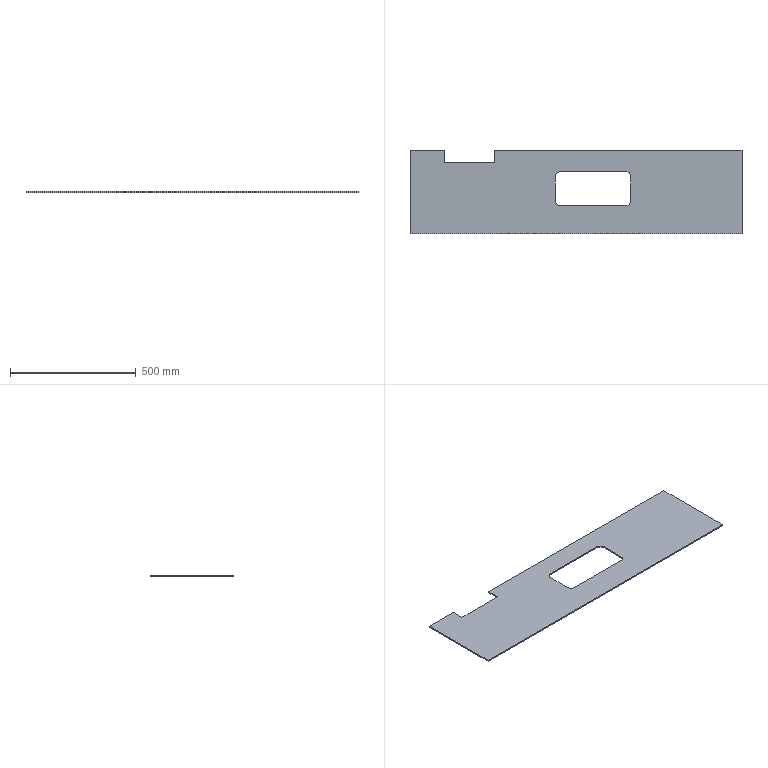Part | STEP file | 1 solid | 18 faces | box 1318 x 331 x 5 mm | volume 1931507 mm3 | plane 14 | cylinder 4 | commonest cylinder face diameters 40 x4
STEP:
#1=CARTESIAN_POINT('',(0.,0.,0.));
#2=DIRECTION('',(0.,0.,1.));
#3=DIRECTION('',(1.,0.,0.));
#4=AXIS2_PLACEMENT_3D('',#1,#2,#3);
#5=CARTESIAN_POINT('',(198.,-893.,0.));
#6=VERTEX_POINT('',#5);
#7=CARTESIAN_POINT('',(-62.,-893.,0.));
#8=VERTEX_POINT('',#7);
#9=CARTESIAN_POINT('',(-62.,-893.,0.));
#10=DIRECTION('',(-1.,0.,0.));
#11=VECTOR('',#10,1.);
#12=LINE('',#9,#11);
#13=CARTESIAN_POINT('',(0.,0.,0.));
#14=DIRECTION('',(0.,0.,-1.));
#15=DIRECTION('',(0.,-1.,0.));
#16=AXIS2_PLACEMENT_3D('',#13,#14,#15);
#17=PLANE('',#16);
#18=CARTESIAN_POINT('',(893.,62.));
#19=DIRECTION('',(0.,1.));
#20=VECTOR('',#19,1.);
#21=LINE('',#18,#20);
#22=(GEOMETRIC_REPRESENTATION_CONTEXT(2)PARAMETRIC_REPRESENTATION_CONTEXT()REPRESENTATION_CONTEXT('',''));
#23=DEFINITIONAL_REPRESENTATION('',(#21),#22);
#24=PCURVE('',#17,#23);
#25=CARTESIAN_POINT('',(-62.,-893.,5.));
#26=DIRECTION('',(0.,1.,0.));
#27=DIRECTION('',(1.,0.,0.));
#28=AXIS2_PLACEMENT_3D('',#25,#26,#27);
#29=PLANE('',#28);
#30=CARTESIAN_POINT('',(0.,5.));
#31=DIRECTION('',(-1.,0.));
#32=VECTOR('',#31,1.);
#33=LINE('',#30,#32);
#34=(GEOMETRIC_REPRESENTATION_CONTEXT(2)PARAMETRIC_REPRESENTATION_CONTEXT()REPRESENTATION_CONTEXT('',''));
#35=DEFINITIONAL_REPRESENTATION('',(#33),#34);
#36=PCURVE('',#29,#35);
#37=SURFACE_CURVE('',#12,(#24,#36),.PCURVE_S1.);
#38=EDGE_CURVE('',#6,#8,#37,.T.);
#39=ORIENTED_EDGE('',*,*,#38,.T.);
#40=CARTESIAN_POINT('',(-82.,-913.,0.));
#41=VERTEX_POINT('',#40);
#42=CARTESIAN_POINT('',(-62.,-913.,0.));
#43=DIRECTION('',(0.,0.,1.));
#44=DIRECTION('',(-1.,0.,0.));
#45=AXIS2_PLACEMENT_3D('',#42,#43,#44);
#46=CIRCLE('',#45,20.);
#47=CARTESIAN_POINT('',(913.,82.));
#48=CARTESIAN_POINT('',(947.641,82.));
#49=CARTESIAN_POINT('',(930.321,52.));
#50=CARTESIAN_POINT('',(913.,22.));
#51=CARTESIAN_POINT('',(895.679,52.));
#52=CARTESIAN_POINT('',(878.359,82.));
#53=CARTESIAN_POINT('',(913.,82.));
#54=(BOUNDED_CURVE()B_SPLINE_CURVE(2,(#47,#48,#49,#50,#51,#52,#53),.UNSPECIFIED.,.T.,.F.)B_SPLINE_CURVE_WITH_KNOTS((1,2,2,2,2,1),(-2.094,0.,2.094,4.189,6.283,8.378),.UNSPECIFIED.)CURVE()GEOMETRIC_REPRESENTATION_ITEM()RATIONAL_B_SPLINE_CURVE((1.,0.5,1.,0.5,1.,0.5,1.))REPRESENTATION_ITEM(''));
#55=(GEOMETRIC_REPRESENTATION_CONTEXT(2)PARAMETRIC_REPRESENTATION_CONTEXT()REPRESENTATION_CONTEXT('',''));
#56=DEFINITIONAL_REPRESENTATION('',(#54),#55);
#57=PCURVE('',#17,#56);
#58=CARTESIAN_POINT('',(-62.,-913.,5.));
#59=DIRECTION('',(0.,0.,-1.));
#60=DIRECTION('',(-1.,0.,0.));
#61=AXIS2_PLACEMENT_3D('',#58,#59,#60);
#62=CYLINDRICAL_SURFACE('',#61,20.);
#63=CARTESIAN_POINT('',(6.283,5.));
#64=DIRECTION('',(-1.,0.));
#65=VECTOR('',#64,1.);
#66=LINE('',#63,#65);
#67=(GEOMETRIC_REPRESENTATION_CONTEXT(2)PARAMETRIC_REPRESENTATION_CONTEXT()REPRESENTATION_CONTEXT('',''));
#68=DEFINITIONAL_REPRESENTATION('',(#66),#67);
#69=PCURVE('',#62,#68);
#70=SURFACE_CURVE('',#46,(#57,#69),.PCURVE_S1.);
#71=EDGE_CURVE('',#8,#41,#70,.T.);
#72=ORIENTED_EDGE('',*,*,#71,.T.);
#73=CARTESIAN_POINT('',(-82.,-1008.,0.));
#74=VERTEX_POINT('',#73);
#75=CARTESIAN_POINT('',(-82.,-913.,0.));
#76=DIRECTION('',(0.,1.,0.));
#77=VECTOR('',#76,1.);
#78=LINE('',#75,#77);
#79=CARTESIAN_POINT('',(913.,82.));
#80=DIRECTION('',(-1.,0.));
#81=VECTOR('',#80,1.);
#82=LINE('',#79,#81);
#83=(GEOMETRIC_REPRESENTATION_CONTEXT(2)PARAMETRIC_REPRESENTATION_CONTEXT()REPRESENTATION_CONTEXT('',''));
#84=DEFINITIONAL_REPRESENTATION('',(#82),#83);
#85=PCURVE('',#17,#84);
#86=CARTESIAN_POINT('',(-82.,-913.,5.));
#87=DIRECTION('',(1.,0.,0.));
#88=DIRECTION('',(0.,1.,0.));
#89=AXIS2_PLACEMENT_3D('',#86,#87,#88);
#90=PLANE('',#89);
#91=CARTESIAN_POINT('',(0.,-5.));
#92=DIRECTION('',(1.,0.));
#93=VECTOR('',#92,1.);
#94=LINE('',#91,#93);
#95=(GEOMETRIC_REPRESENTATION_CONTEXT(2)PARAMETRIC_REPRESENTATION_CONTEXT()REPRESENTATION_CONTEXT('',''));
#96=DEFINITIONAL_REPRESENTATION('',(#94),#95);
#97=PCURVE('',#90,#96);
#98=SURFACE_CURVE('',#78,(#85,#97),.PCURVE_S1.);
#99=EDGE_CURVE('',#74,#41,#98,.T.);
#100=ORIENTED_EDGE('',*,*,#99,.F.);
#101=CARTESIAN_POINT('',(-62.,-1028.,0.));
#102=VERTEX_POINT('',#101);
#103=CARTESIAN_POINT('',(-62.,-1008.,0.));
#104=DIRECTION('',(0.,0.,1.));
#105=DIRECTION('',(-1.,0.,0.));
#106=AXIS2_PLACEMENT_3D('',#103,#104,#105);
#107=CIRCLE('',#106,20.);
#108=CARTESIAN_POINT('',(1008.,82.));
#109=CARTESIAN_POINT('',(1042.641,82.));
#110=CARTESIAN_POINT('',(1025.321,52.));
#111=CARTESIAN_POINT('',(1008.,22.));
#112=CARTESIAN_POINT('',(990.679,52.));
#113=CARTESIAN_POINT('',(973.359,82.));
#114=CARTESIAN_POINT('',(1008.,82.));
#115=(BOUNDED_CURVE()B_SPLINE_CURVE(2,(#108,#109,#110,#111,#112,#113,#114),.UNSPECIFIED.,.T.,.F.)B_SPLINE_CURVE_WITH_KNOTS((1,2,2,2,2,1),(-2.094,0.,2.094,4.189,6.283,8.378),.UNSPECIFIED.)CURVE()GEOMETRIC_REPRESENTATION_ITEM()RATIONAL_B_SPLINE_CURVE((1.,0.5,1.,0.5,1.,0.5,1.))REPRESENTATION_ITEM(''));
#116=(GEOMETRIC_REPRESENTATION_CONTEXT(2)PARAMETRIC_REPRESENTATION_CONTEXT()REPRESENTATION_CONTEXT('',''));
#117=DEFINITIONAL_REPRESENTATION('',(#115),#116);
#118=PCURVE('',#17,#117);
#119=CARTESIAN_POINT('',(-62.,-1008.,5.));
#120=DIRECTION('',(0.,0.,-1.));
#121=DIRECTION('',(-1.,0.,0.));
#122=AXIS2_PLACEMENT_3D('',#119,#120,#121);
#123=CYLINDRICAL_SURFACE('',#122,20.);
#124=CARTESIAN_POINT('',(6.283,5.));
#125=DIRECTION('',(-1.,0.));
#126=VECTOR('',#125,1.);
#127=LINE('',#124,#126);
#128=(GEOMETRIC_REPRESENTATION_CONTEXT(2)PARAMETRIC_REPRESENTATION_CONTEXT()REPRESENTATION_CONTEXT('',''));
#129=DEFINITIONAL_REPRESENTATION('',(#127),#128);
#130=PCURVE('',#123,#129);
#131=SURFACE_CURVE('',#107,(#118,#130),.PCURVE_S1.);
#132=EDGE_CURVE('',#74,#102,#131,.T.);
#133=ORIENTED_EDGE('',*,*,#132,.T.);
#134=CARTESIAN_POINT('',(198.,-1028.,0.));
#135=VERTEX_POINT('',#134);
#136=CARTESIAN_POINT('',(-62.,-1028.,0.));
#137=DIRECTION('',(-1.,0.,0.));
#138=VECTOR('',#137,1.);
#139=LINE('',#136,#138);
#140=CARTESIAN_POINT('',(1028.,62.));
#141=DIRECTION('',(0.,1.));
#142=VECTOR('',#141,1.);
#143=LINE('',#140,#142);
#144=(GEOMETRIC_REPRESENTATION_CONTEXT(2)PARAMETRIC_REPRESENTATION_CONTEXT()REPRESENTATION_CONTEXT('',''));
#145=DEFINITIONAL_REPRESENTATION('',(#143),#144);
#146=PCURVE('',#17,#145);
#147=CARTESIAN_POINT('',(-62.,-1028.,5.));
#148=DIRECTION('',(0.,1.,0.));
#149=DIRECTION('',(1.,0.,0.));
#150=AXIS2_PLACEMENT_3D('',#147,#148,#149);
#151=PLANE('',#150);
#152=CARTESIAN_POINT('',(0.,5.));
#153=DIRECTION('',(-1.,0.));
#154=VECTOR('',#153,1.);
#155=LINE('',#152,#154);
#156=(GEOMETRIC_REPRESENTATION_CONTEXT(2)PARAMETRIC_REPRESENTATION_CONTEXT()REPRESENTATION_CONTEXT('',''));
#157=DEFINITIONAL_REPRESENTATION('',(#155),#156);
#158=PCURVE('',#151,#157);
#159=SURFACE_CURVE('',#139,(#146,#158),.PCURVE_S1.);
#160=EDGE_CURVE('',#135,#102,#159,.T.);
#161=ORIENTED_EDGE('',*,*,#160,.F.);
#162=CARTESIAN_POINT('',(218.,-1008.,0.));
#163=VERTEX_POINT('',#162);
#164=CARTESIAN_POINT('',(198.,-1008.,0.));
#165=DIRECTION('',(0.,0.,1.));
#166=DIRECTION('',(-1.,0.,0.));
#167=AXIS2_PLACEMENT_3D('',#164,#165,#166);
#168=CIRCLE('',#167,20.);
#169=CARTESIAN_POINT('',(1008.,-178.));
#170=CARTESIAN_POINT('',(1042.641,-178.));
#171=CARTESIAN_POINT('',(1025.321,-208.));
#172=CARTESIAN_POINT('',(1008.,-238.));
#173=CARTESIAN_POINT('',(990.679,-208.));
#174=CARTESIAN_POINT('',(973.359,-178.));
#175=CARTESIAN_POINT('',(1008.,-178.));
#176=(BOUNDED_CURVE()B_SPLINE_CURVE(2,(#169,#170,#171,#172,#173,#174,#175),.UNSPECIFIED.,.T.,.F.)B_SPLINE_CURVE_WITH_KNOTS((1,2,2,2,2,1),(-2.094,0.,2.094,4.189,6.283,8.378),.UNSPECIFIED.)CURVE()GEOMETRIC_REPRESENTATION_ITEM()RATIONAL_B_SPLINE_CURVE((1.,0.5,1.,0.5,1.,0.5,1.))REPRESENTATION_ITEM(''));
#177=(GEOMETRIC_REPRESENTATION_CONTEXT(2)PARAMETRIC_REPRESENTATION_CONTEXT()REPRESENTATION_CONTEXT('',''));
#178=DEFINITIONAL_REPRESENTATION('',(#176),#177);
#179=PCURVE('',#17,#178);
#180=CARTESIAN_POINT('',(198.,-1008.,5.));
#181=DIRECTION('',(0.,0.,-1.));
#182=DIRECTION('',(-1.,0.,0.));
#183=AXIS2_PLACEMENT_3D('',#180,#181,#182);
#184=CYLINDRICAL_SURFACE('',#183,20.);
#185=CARTESIAN_POINT('',(6.283,5.));
#186=DIRECTION('',(-1.,0.));
#187=VECTOR('',#186,1.);
#188=LINE('',#185,#187);
#189=(GEOMETRIC_REPRESENTATION_CONTEXT(2)PARAMETRIC_REPRESENTATION_CONTEXT()REPRESENTATION_CONTEXT('',''));
#190=DEFINITIONAL_REPRESENTATION('',(#188),#189);
#191=PCURVE('',#184,#190);
#192=SURFACE_CURVE('',#168,(#179,#191),.PCURVE_S1.);
#193=EDGE_CURVE('',#135,#163,#192,.T.);
#194=ORIENTED_EDGE('',*,*,#193,.T.);
#195=CARTESIAN_POINT('',(218.,-913.,0.));
#196=VERTEX_POINT('',#195);
#197=CARTESIAN_POINT('',(218.,-913.,0.));
#198=DIRECTION('',(0.,1.,0.));
#199=VECTOR('',#198,1.);
#200=LINE('',#197,#199);
#201=CARTESIAN_POINT('',(913.,-218.));
#202=DIRECTION('',(-1.,0.));
#203=VECTOR('',#202,1.);
#204=LINE('',#201,#203);
#205=(GEOMETRIC_REPRESENTATION_CONTEXT(2)PARAMETRIC_REPRESENTATION_CONTEXT()REPRESENTATION_CONTEXT('',''));
#206=DEFINITIONAL_REPRESENTATION('',(#204),#205);
#207=PCURVE('',#17,#206);
#208=CARTESIAN_POINT('',(218.,-913.,5.));
#209=DIRECTION('',(1.,0.,0.));
#210=DIRECTION('',(0.,1.,0.));
#211=AXIS2_PLACEMENT_3D('',#208,#209,#210);
#212=PLANE('',#211);
#213=CARTESIAN_POINT('',(0.,-5.));
#214=DIRECTION('',(1.,0.));
#215=VECTOR('',#214,1.);
#216=LINE('',#213,#215);
#217=(GEOMETRIC_REPRESENTATION_CONTEXT(2)PARAMETRIC_REPRESENTATION_CONTEXT()REPRESENTATION_CONTEXT('',''));
#218=DEFINITIONAL_REPRESENTATION('',(#216),#217);
#219=PCURVE('',#212,#218);
#220=SURFACE_CURVE('',#200,(#207,#219),.PCURVE_S1.);
#221=EDGE_CURVE('',#163,#196,#220,.T.);
#222=ORIENTED_EDGE('',*,*,#221,.T.);
#223=CARTESIAN_POINT('',(198.,-913.,0.));
#224=DIRECTION('',(0.,0.,1.));
#225=DIRECTION('',(-1.,0.,0.));
#226=AXIS2_PLACEMENT_3D('',#223,#224,#225);
#227=CIRCLE('',#226,20.);
#228=CARTESIAN_POINT('',(913.,-178.));
#229=CARTESIAN_POINT('',(947.641,-178.));
#230=CARTESIAN_POINT('',(930.321,-208.));
#231=CARTESIAN_POINT('',(913.,-238.));
#232=CARTESIAN_POINT('',(895.679,-208.));
#233=CARTESIAN_POINT('',(878.359,-178.));
#234=CARTESIAN_POINT('',(913.,-178.));
#235=(BOUNDED_CURVE()B_SPLINE_CURVE(2,(#228,#229,#230,#231,#232,#233,#234),.UNSPECIFIED.,.T.,.F.)B_SPLINE_CURVE_WITH_KNOTS((1,2,2,2,2,1),(-2.094,0.,2.094,4.189,6.283,8.378),.UNSPECIFIED.)CURVE()GEOMETRIC_REPRESENTATION_ITEM()RATIONAL_B_SPLINE_CURVE((1.,0.5,1.,0.5,1.,0.5,1.))REPRESENTATION_ITEM(''));
#236=(GEOMETRIC_REPRESENTATION_CONTEXT(2)PARAMETRIC_REPRESENTATION_CONTEXT()REPRESENTATION_CONTEXT('',''));
#237=DEFINITIONAL_REPRESENTATION('',(#235),#236);
#238=PCURVE('',#17,#237);
#239=CARTESIAN_POINT('',(198.,-913.,5.));
#240=DIRECTION('',(0.,0.,-1.));
#241=DIRECTION('',(-1.,0.,0.));
#242=AXIS2_PLACEMENT_3D('',#239,#240,#241);
#243=CYLINDRICAL_SURFACE('',#242,20.);
#244=CARTESIAN_POINT('',(6.283,5.));
#245=DIRECTION('',(-1.,0.));
#246=VECTOR('',#245,1.);
#247=LINE('',#244,#246);
#248=(GEOMETRIC_REPRESENTATION_CONTEXT(2)PARAMETRIC_REPRESENTATION_CONTEXT()REPRESENTATION_CONTEXT('',''));
#249=DEFINITIONAL_REPRESENTATION('',(#247),#248);
#250=PCURVE('',#243,#249);
#251=SURFACE_CURVE('',#227,(#238,#250),.PCURVE_S1.);
#252=EDGE_CURVE('',#196,#6,#251,.T.);
#253=ORIENTED_EDGE('',*,*,#252,.T.);
#254=EDGE_LOOP('',(#39,#72,#100,#133,#161,#194,#222,#253));
#255=FACE_BOUND('',#254,.T.);
#256=CARTESIAN_POINT('',(-324.,-857.,0.));
#257=VERTEX_POINT('',#256);
#258=CARTESIAN_POINT('',(-524.,-857.,0.));
#259=VERTEX_POINT('',#258);
#260=CARTESIAN_POINT('',(-524.,-857.,0.));
#261=DIRECTION('',(-1.,0.,0.));
#262=VECTOR('',#261,1.);
#263=LINE('',#260,#262);
#264=CARTESIAN_POINT('',(857.,524.));
#265=DIRECTION('',(0.,1.));
#266=VECTOR('',#265,1.);
#267=LINE('',#264,#266);
#268=(GEOMETRIC_REPRESENTATION_CONTEXT(2)PARAMETRIC_REPRESENTATION_CONTEXT()REPRESENTATION_CONTEXT('',''));
#269=DEFINITIONAL_REPRESENTATION('',(#267),#268);
#270=PCURVE('',#17,#269);
#271=CARTESIAN_POINT('',(-524.,-857.,5.));
#272=DIRECTION('',(0.,1.,0.));
#273=DIRECTION('',(1.,0.,0.));
#274=AXIS2_PLACEMENT_3D('',#271,#272,#273);
#275=PLANE('',#274);
#276=CARTESIAN_POINT('',(0.,5.));
#277=DIRECTION('',(-1.,0.));
#278=VECTOR('',#277,1.);
#279=LINE('',#276,#278);
#280=(GEOMETRIC_REPRESENTATION_CONTEXT(2)PARAMETRIC_REPRESENTATION_CONTEXT()REPRESENTATION_CONTEXT('',''));
#281=DEFINITIONAL_REPRESENTATION('',(#279),#280);
#282=PCURVE('',#275,#281);
#283=SURFACE_CURVE('',#263,(#270,#282),.PCURVE_S1.);
#284=EDGE_CURVE('',#257,#259,#283,.T.);
#285=ORIENTED_EDGE('',*,*,#284,.F.);
#286=CARTESIAN_POINT('',(-324.,-808.,0.));
#287=VERTEX_POINT('',#286);
#288=CARTESIAN_POINT('',(-324.,-857.,0.));
#289=DIRECTION('',(0.,-1.,0.));
#290=VECTOR('',#289,1.);
#291=LINE('',#288,#290);
#292=CARTESIAN_POINT('',(857.,324.));
#293=DIRECTION('',(1.,0.));
#294=VECTOR('',#293,1.);
#295=LINE('',#292,#294);
#296=(GEOMETRIC_REPRESENTATION_CONTEXT(2)PARAMETRIC_REPRESENTATION_CONTEXT()REPRESENTATION_CONTEXT('',''));
#297=DEFINITIONAL_REPRESENTATION('',(#295),#296);
#298=PCURVE('',#17,#297);
#299=CARTESIAN_POINT('',(-324.,-857.,5.));
#300=DIRECTION('',(-1.,0.,0.));
#301=DIRECTION('',(0.,0.,1.));
#302=AXIS2_PLACEMENT_3D('',#299,#300,#301);
#303=PLANE('',#302);
#304=CARTESIAN_POINT('',(-5.,0.));
#305=DIRECTION('',(0.,-1.));
#306=VECTOR('',#305,1.);
#307=LINE('',#304,#306);
#308=(GEOMETRIC_REPRESENTATION_CONTEXT(2)PARAMETRIC_REPRESENTATION_CONTEXT()REPRESENTATION_CONTEXT('',''));
#309=DEFINITIONAL_REPRESENTATION('',(#307),#308);
#310=PCURVE('',#303,#309);
#311=SURFACE_CURVE('',#291,(#298,#310),.PCURVE_S1.);
#312=EDGE_CURVE('',#287,#257,#311,.T.);
#313=ORIENTED_EDGE('',*,*,#312,.F.);
#314=CARTESIAN_POINT('',(659.,-808.,0.));
#315=VERTEX_POINT('',#314);
#316=CARTESIAN_POINT('',(-324.,-808.,0.));
#317=DIRECTION('',(-1.,0.,0.));
#318=VECTOR('',#317,1.);
#319=LINE('',#316,#318);
#320=CARTESIAN_POINT('',(808.,324.));
#321=DIRECTION('',(0.,1.));
#322=VECTOR('',#321,1.);
#323=LINE('',#320,#322);
#324=(GEOMETRIC_REPRESENTATION_CONTEXT(2)PARAMETRIC_REPRESENTATION_CONTEXT()REPRESENTATION_CONTEXT('',''));
#325=DEFINITIONAL_REPRESENTATION('',(#323),#324);
#326=PCURVE('',#17,#325);
#327=CARTESIAN_POINT('',(-324.,-808.,5.));
#328=DIRECTION('',(0.,1.,0.));
#329=DIRECTION('',(1.,0.,0.));
#330=AXIS2_PLACEMENT_3D('',#327,#328,#329);
#331=PLANE('',#330);
#332=CARTESIAN_POINT('',(0.,5.));
#333=DIRECTION('',(-1.,0.));
#334=VECTOR('',#333,1.);
#335=LINE('',#332,#334);
#336=(GEOMETRIC_REPRESENTATION_CONTEXT(2)PARAMETRIC_REPRESENTATION_CONTEXT()REPRESENTATION_CONTEXT('',''));
#337=DEFINITIONAL_REPRESENTATION('',(#335),#336);
#338=PCURVE('',#331,#337);
#339=SURFACE_CURVE('',#319,(#326,#338),.PCURVE_S1.);
#340=EDGE_CURVE('',#315,#287,#339,.T.);
#341=ORIENTED_EDGE('',*,*,#340,.F.);
#342=CARTESIAN_POINT('',(659.,-1139.,0.));
#343=VERTEX_POINT('',#342);
#344=CARTESIAN_POINT('',(659.,-808.,0.));
#345=DIRECTION('',(0.,1.,0.));
#346=VECTOR('',#345,1.);
#347=LINE('',#344,#346);
#348=CARTESIAN_POINT('',(808.,-659.));
#349=DIRECTION('',(-1.,0.));
#350=VECTOR('',#349,1.);
#351=LINE('',#348,#350);
#352=(GEOMETRIC_REPRESENTATION_CONTEXT(2)PARAMETRIC_REPRESENTATION_CONTEXT()REPRESENTATION_CONTEXT('',''));
#353=DEFINITIONAL_REPRESENTATION('',(#351),#352);
#354=PCURVE('',#17,#353);
#355=CARTESIAN_POINT('',(659.,-808.,5.));
#356=DIRECTION('',(1.,0.,0.));
#357=DIRECTION('',(0.,-1.,0.));
#358=AXIS2_PLACEMENT_3D('',#355,#356,#357);
#359=PLANE('',#358);
#360=CARTESIAN_POINT('',(0.,5.));
#361=DIRECTION('',(-1.,0.));
#362=VECTOR('',#361,1.);
#363=LINE('',#360,#362);
#364=(GEOMETRIC_REPRESENTATION_CONTEXT(2)PARAMETRIC_REPRESENTATION_CONTEXT()REPRESENTATION_CONTEXT('',''));
#365=DEFINITIONAL_REPRESENTATION('',(#363),#364);
#366=PCURVE('',#359,#365);
#367=SURFACE_CURVE('',#347,(#354,#366),.PCURVE_S1.);
#368=EDGE_CURVE('',#343,#315,#367,.T.);
#369=ORIENTED_EDGE('',*,*,#368,.F.);
#370=CARTESIAN_POINT('',(-659.,-1139.,0.));
#371=VERTEX_POINT('',#370);
#372=CARTESIAN_POINT('',(-659.,-1139.,0.));
#373=DIRECTION('',(-1.,0.,0.));
#374=VECTOR('',#373,1.);
#375=LINE('',#372,#374);
#376=CARTESIAN_POINT('',(1139.,659.));
#377=DIRECTION('',(0.,1.));
#378=VECTOR('',#377,1.);
#379=LINE('',#376,#378);
#380=(GEOMETRIC_REPRESENTATION_CONTEXT(2)PARAMETRIC_REPRESENTATION_CONTEXT()REPRESENTATION_CONTEXT('',''));
#381=DEFINITIONAL_REPRESENTATION('',(#379),#380);
#382=PCURVE('',#17,#381);
#383=CARTESIAN_POINT('',(-659.,-1139.,5.));
#384=DIRECTION('',(0.,1.,0.));
#385=DIRECTION('',(1.,0.,0.));
#386=AXIS2_PLACEMENT_3D('',#383,#384,#385);
#387=PLANE('',#386);
#388=CARTESIAN_POINT('',(0.,5.));
#389=DIRECTION('',(-1.,0.));
#390=VECTOR('',#389,1.);
#391=LINE('',#388,#390);
#392=(GEOMETRIC_REPRESENTATION_CONTEXT(2)PARAMETRIC_REPRESENTATION_CONTEXT()REPRESENTATION_CONTEXT('',''));
#393=DEFINITIONAL_REPRESENTATION('',(#391),#392);
#394=PCURVE('',#387,#393);
#395=SURFACE_CURVE('',#375,(#382,#394),.PCURVE_S1.);
#396=EDGE_CURVE('',#343,#371,#395,.T.);
#397=ORIENTED_EDGE('',*,*,#396,.T.);
#398=CARTESIAN_POINT('',(-659.,-808.,0.));
#399=VERTEX_POINT('',#398);
#400=CARTESIAN_POINT('',(-659.,-808.,0.));
#401=DIRECTION('',(0.,1.,0.));
#402=VECTOR('',#401,1.);
#403=LINE('',#400,#402);
#404=CARTESIAN_POINT('',(808.,659.));
#405=DIRECTION('',(-1.,0.));
#406=VECTOR('',#405,1.);
#407=LINE('',#404,#406);
#408=(GEOMETRIC_REPRESENTATION_CONTEXT(2)PARAMETRIC_REPRESENTATION_CONTEXT()REPRESENTATION_CONTEXT('',''));
#409=DEFINITIONAL_REPRESENTATION('',(#407),#408);
#410=PCURVE('',#17,#409);
#411=CARTESIAN_POINT('',(-659.,-808.,5.));
#412=DIRECTION('',(1.,0.,0.));
#413=DIRECTION('',(0.,1.,0.));
#414=AXIS2_PLACEMENT_3D('',#411,#412,#413);
#415=PLANE('',#414);
#416=CARTESIAN_POINT('',(0.,-5.));
#417=DIRECTION('',(1.,0.));
#418=VECTOR('',#417,1.);
#419=LINE('',#416,#418);
#420=(GEOMETRIC_REPRESENTATION_CONTEXT(2)PARAMETRIC_REPRESENTATION_CONTEXT()REPRESENTATION_CONTEXT('',''));
#421=DEFINITIONAL_REPRESENTATION('',(#419),#420);
#422=PCURVE('',#415,#421);
#423=SURFACE_CURVE('',#403,(#410,#422),.PCURVE_S1.);
#424=EDGE_CURVE('',#371,#399,#423,.T.);
#425=ORIENTED_EDGE('',*,*,#424,.T.);
#426=CARTESIAN_POINT('',(-524.,-808.,0.));
#427=VERTEX_POINT('',#426);
#428=CARTESIAN_POINT('',(-659.,-808.,0.));
#429=DIRECTION('',(-1.,0.,0.));
#430=VECTOR('',#429,1.);
#431=LINE('',#428,#430);
#432=CARTESIAN_POINT('',(808.,659.));
#433=DIRECTION('',(0.,1.));
#434=VECTOR('',#433,1.);
#435=LINE('',#432,#434);
#436=(GEOMETRIC_REPRESENTATION_CONTEXT(2)PARAMETRIC_REPRESENTATION_CONTEXT()REPRESENTATION_CONTEXT('',''));
#437=DEFINITIONAL_REPRESENTATION('',(#435),#436);
#438=PCURVE('',#17,#437);
#439=CARTESIAN_POINT('',(-659.,-808.,5.));
#440=DIRECTION('',(0.,1.,0.));
#441=DIRECTION('',(1.,0.,0.));
#442=AXIS2_PLACEMENT_3D('',#439,#440,#441);
#443=PLANE('',#442);
#444=CARTESIAN_POINT('',(0.,5.));
#445=DIRECTION('',(-1.,0.));
#446=VECTOR('',#445,1.);
#447=LINE('',#444,#446);
#448=(GEOMETRIC_REPRESENTATION_CONTEXT(2)PARAMETRIC_REPRESENTATION_CONTEXT()REPRESENTATION_CONTEXT('',''));
#449=DEFINITIONAL_REPRESENTATION('',(#447),#448);
#450=PCURVE('',#443,#449);
#451=SURFACE_CURVE('',#431,(#438,#450),.PCURVE_S1.);
#452=EDGE_CURVE('',#427,#399,#451,.T.);
#453=ORIENTED_EDGE('',*,*,#452,.F.);
#454=CARTESIAN_POINT('',(-524.,-857.,0.));
#455=DIRECTION('',(0.,-1.,0.));
#456=VECTOR('',#455,1.);
#457=LINE('',#454,#456);
#458=CARTESIAN_POINT('',(857.,524.));
#459=DIRECTION('',(1.,0.));
#460=VECTOR('',#459,1.);
#461=LINE('',#458,#460);
#462=(GEOMETRIC_REPRESENTATION_CONTEXT(2)PARAMETRIC_REPRESENTATION_CONTEXT()REPRESENTATION_CONTEXT('',''));
#463=DEFINITIONAL_REPRESENTATION('',(#461),#462);
#464=PCURVE('',#17,#463);
#465=CARTESIAN_POINT('',(-524.,-857.,5.));
#466=DIRECTION('',(-1.,0.,0.));
#467=DIRECTION('',(0.,0.,1.));
#468=AXIS2_PLACEMENT_3D('',#465,#466,#467);
#469=PLANE('',#468);
#470=CARTESIAN_POINT('',(-5.,0.));
#471=DIRECTION('',(0.,-1.));
#472=VECTOR('',#471,1.);
#473=LINE('',#470,#472);
#474=(GEOMETRIC_REPRESENTATION_CONTEXT(2)PARAMETRIC_REPRESENTATION_CONTEXT()REPRESENTATION_CONTEXT('',''));
#475=DEFINITIONAL_REPRESENTATION('',(#473),#474);
#476=PCURVE('',#469,#475);
#477=SURFACE_CURVE('',#457,(#464,#476),.PCURVE_S1.);
#478=EDGE_CURVE('',#427,#259,#477,.T.);
#479=ORIENTED_EDGE('',*,*,#478,.T.);
#480=EDGE_LOOP('',(#285,#313,#341,#369,#397,#425,#453,#479));
#481=FACE_BOUND('',#480,.T.);
#482=ADVANCED_FACE('',(#255,#481),#17,.T.);
#483=CARTESIAN_POINT('',(659.,-808.,5.));
#484=VERTEX_POINT('',#483);
#485=CARTESIAN_POINT('',(659.,-1139.,5.));
#486=VERTEX_POINT('',#485);
#487=CARTESIAN_POINT('',(659.,0.,5.));
#488=DIRECTION('',(0.,-1.,0.));
#489=VECTOR('',#488,1.);
#490=LINE('',#487,#489);
#491=CARTESIAN_POINT('',(-808.,0.));
#492=DIRECTION('',(1.,0.));
#493=VECTOR('',#492,1.);
#494=LINE('',#491,#493);
#495=(GEOMETRIC_REPRESENTATION_CONTEXT(2)PARAMETRIC_REPRESENTATION_CONTEXT()REPRESENTATION_CONTEXT('',''));
#496=DEFINITIONAL_REPRESENTATION('',(#494),#495);
#497=PCURVE('',#359,#496);
#498=CARTESIAN_POINT('',(0.,0.,5.));
#499=DIRECTION('',(0.,0.,-1.));
#500=DIRECTION('',(0.,-1.,0.));
#501=AXIS2_PLACEMENT_3D('',#498,#499,#500);
#502=PLANE('',#501);
#503=CARTESIAN_POINT('',(0.,-659.));
#504=DIRECTION('',(1.,0.));
#505=VECTOR('',#504,1.);
#506=LINE('',#503,#505);
#507=(GEOMETRIC_REPRESENTATION_CONTEXT(2)PARAMETRIC_REPRESENTATION_CONTEXT()REPRESENTATION_CONTEXT('',''));
#508=DEFINITIONAL_REPRESENTATION('',(#506),#507);
#509=PCURVE('',#502,#508);
#510=SURFACE_CURVE('',#490,(#497,#509),.PCURVE_S1.);
#511=EDGE_CURVE('',#484,#486,#510,.T.);
#512=ORIENTED_EDGE('',*,*,#511,.T.);
#513=CARTESIAN_POINT('',(659.,-1139.,5.));
#514=DIRECTION('',(0.,0.,-1.));
#515=VECTOR('',#514,1.);
#516=LINE('',#513,#515);
#517=CARTESIAN_POINT('',(331.,0.));
#518=DIRECTION('',(0.,1.));
#519=VECTOR('',#518,1.);
#520=LINE('',#517,#519);
#521=(GEOMETRIC_REPRESENTATION_CONTEXT(2)PARAMETRIC_REPRESENTATION_CONTEXT()REPRESENTATION_CONTEXT('',''));
#522=DEFINITIONAL_REPRESENTATION('',(#520),#521);
#523=PCURVE('',#359,#522);
#524=CARTESIAN_POINT('',(1318.,0.));
#525=DIRECTION('',(0.,1.));
#526=VECTOR('',#525,1.);
#527=LINE('',#524,#526);
#528=(GEOMETRIC_REPRESENTATION_CONTEXT(2)PARAMETRIC_REPRESENTATION_CONTEXT()REPRESENTATION_CONTEXT('',''));
#529=DEFINITIONAL_REPRESENTATION('',(#527),#528);
#530=PCURVE('',#387,#529);
#531=SURFACE_CURVE('',#516,(#523,#530),.PCURVE_S1.);
#532=EDGE_CURVE('',#486,#343,#531,.T.);
#533=ORIENTED_EDGE('',*,*,#532,.T.);
#534=ORIENTED_EDGE('',*,*,#368,.T.);
#535=CARTESIAN_POINT('',(659.,-808.,5.));
#536=DIRECTION('',(0.,0.,-1.));
#537=VECTOR('',#536,1.);
#538=LINE('',#535,#537);
#539=CARTESIAN_POINT('',(0.,0.));
#540=DIRECTION('',(0.,1.));
#541=VECTOR('',#540,1.);
#542=LINE('',#539,#541);
#543=(GEOMETRIC_REPRESENTATION_CONTEXT(2)PARAMETRIC_REPRESENTATION_CONTEXT()REPRESENTATION_CONTEXT('',''));
#544=DEFINITIONAL_REPRESENTATION('',(#542),#543);
#545=PCURVE('',#359,#544);
#546=CARTESIAN_POINT('',(983.,0.));
#547=DIRECTION('',(0.,1.));
#548=VECTOR('',#547,1.);
#549=LINE('',#546,#548);
#550=(GEOMETRIC_REPRESENTATION_CONTEXT(2)PARAMETRIC_REPRESENTATION_CONTEXT()REPRESENTATION_CONTEXT('',''));
#551=DEFINITIONAL_REPRESENTATION('',(#549),#550);
#552=PCURVE('',#331,#551);
#553=SURFACE_CURVE('',#538,(#545,#552),.PCURVE_S1.);
#554=EDGE_CURVE('',#484,#315,#553,.T.);
#555=ORIENTED_EDGE('',*,*,#554,.F.);
#556=EDGE_LOOP('',(#512,#533,#534,#555));
#557=FACE_BOUND('',#556,.T.);
#558=ADVANCED_FACE('',(#557),#359,.T.);
#559=ORIENTED_EDGE('',*,*,#532,.F.);
#560=CARTESIAN_POINT('',(-659.,-1139.,5.));
#561=VERTEX_POINT('',#560);
#562=CARTESIAN_POINT('',(0.,-1139.,5.));
#563=DIRECTION('',(-1.,0.,0.));
#564=VECTOR('',#563,1.);
#565=LINE('',#562,#564);
#566=CARTESIAN_POINT('',(659.,0.));
#567=DIRECTION('',(-1.,0.));
#568=VECTOR('',#567,1.);
#569=LINE('',#566,#568);
#570=(GEOMETRIC_REPRESENTATION_CONTEXT(2)PARAMETRIC_REPRESENTATION_CONTEXT()REPRESENTATION_CONTEXT('',''));
#571=DEFINITIONAL_REPRESENTATION('',(#569),#570);
#572=PCURVE('',#387,#571);
#573=CARTESIAN_POINT('',(1139.,0.));
#574=DIRECTION('',(0.,1.));
#575=VECTOR('',#574,1.);
#576=LINE('',#573,#575);
#577=(GEOMETRIC_REPRESENTATION_CONTEXT(2)PARAMETRIC_REPRESENTATION_CONTEXT()REPRESENTATION_CONTEXT('',''));
#578=DEFINITIONAL_REPRESENTATION('',(#576),#577);
#579=PCURVE('',#502,#578);
#580=SURFACE_CURVE('',#565,(#572,#579),.PCURVE_S1.);
#581=EDGE_CURVE('',#486,#561,#580,.T.);
#582=ORIENTED_EDGE('',*,*,#581,.T.);
#583=CARTESIAN_POINT('',(-659.,-1139.,5.));
#584=DIRECTION('',(0.,0.,-1.));
#585=VECTOR('',#584,1.);
#586=LINE('',#583,#585);
#587=CARTESIAN_POINT('',(0.,0.));
#588=DIRECTION('',(0.,1.));
#589=VECTOR('',#588,1.);
#590=LINE('',#587,#589);
#591=(GEOMETRIC_REPRESENTATION_CONTEXT(2)PARAMETRIC_REPRESENTATION_CONTEXT()REPRESENTATION_CONTEXT('',''));
#592=DEFINITIONAL_REPRESENTATION('',(#590),#591);
#593=PCURVE('',#387,#592);
#594=CARTESIAN_POINT('',(-331.,0.));
#595=DIRECTION('',(0.,-1.));
#596=VECTOR('',#595,1.);
#597=LINE('',#594,#596);
#598=(GEOMETRIC_REPRESENTATION_CONTEXT(2)PARAMETRIC_REPRESENTATION_CONTEXT()REPRESENTATION_CONTEXT('',''));
#599=DEFINITIONAL_REPRESENTATION('',(#597),#598);
#600=PCURVE('',#415,#599);
#601=SURFACE_CURVE('',#586,(#593,#600),.PCURVE_S1.);
#602=EDGE_CURVE('',#561,#371,#601,.T.);
#603=ORIENTED_EDGE('',*,*,#602,.T.);
#604=ORIENTED_EDGE('',*,*,#396,.F.);
#605=EDGE_LOOP('',(#559,#582,#603,#604));
#606=FACE_BOUND('',#605,.T.);
#607=ADVANCED_FACE('',(#606),#387,.F.);
#608=ORIENTED_EDGE('',*,*,#602,.F.);
#609=CARTESIAN_POINT('',(-659.,-808.,5.));
#610=VERTEX_POINT('',#609);
#611=CARTESIAN_POINT('',(-659.,0.,5.));
#612=DIRECTION('',(0.,1.,0.));
#613=VECTOR('',#612,1.);
#614=LINE('',#611,#613);
#615=CARTESIAN_POINT('',(808.,0.));
#616=DIRECTION('',(1.,0.));
#617=VECTOR('',#616,1.);
#618=LINE('',#615,#617);
#619=(GEOMETRIC_REPRESENTATION_CONTEXT(2)PARAMETRIC_REPRESENTATION_CONTEXT()REPRESENTATION_CONTEXT('',''));
#620=DEFINITIONAL_REPRESENTATION('',(#618),#619);
#621=PCURVE('',#415,#620);
#622=CARTESIAN_POINT('',(0.,659.));
#623=DIRECTION('',(-1.,0.));
#624=VECTOR('',#623,1.);
#625=LINE('',#622,#624);
#626=(GEOMETRIC_REPRESENTATION_CONTEXT(2)PARAMETRIC_REPRESENTATION_CONTEXT()REPRESENTATION_CONTEXT('',''));
#627=DEFINITIONAL_REPRESENTATION('',(#625),#626);
#628=PCURVE('',#502,#627);
#629=SURFACE_CURVE('',#614,(#621,#628),.PCURVE_S1.);
#630=EDGE_CURVE('',#561,#610,#629,.T.);
#631=ORIENTED_EDGE('',*,*,#630,.T.);
#632=CARTESIAN_POINT('',(-659.,-808.,5.));
#633=DIRECTION('',(0.,0.,1.));
#634=VECTOR('',#633,1.);
#635=LINE('',#632,#634);
#636=CARTESIAN_POINT('',(0.,0.));
#637=DIRECTION('',(0.,1.));
#638=VECTOR('',#637,1.);
#639=LINE('',#636,#638);
#640=(GEOMETRIC_REPRESENTATION_CONTEXT(2)PARAMETRIC_REPRESENTATION_CONTEXT()REPRESENTATION_CONTEXT('',''));
#641=DEFINITIONAL_REPRESENTATION('',(#639),#640);
#642=PCURVE('',#415,#641);
#643=CARTESIAN_POINT('',(0.,0.));
#644=DIRECTION('',(0.,-1.));
#645=VECTOR('',#644,1.);
#646=LINE('',#643,#645);
#647=(GEOMETRIC_REPRESENTATION_CONTEXT(2)PARAMETRIC_REPRESENTATION_CONTEXT()REPRESENTATION_CONTEXT('',''));
#648=DEFINITIONAL_REPRESENTATION('',(#646),#647);
#649=PCURVE('',#443,#648);
#650=SURFACE_CURVE('',#635,(#642,#649),.PCURVE_S1.);
#651=EDGE_CURVE('',#399,#610,#650,.T.);
#652=ORIENTED_EDGE('',*,*,#651,.F.);
#653=ORIENTED_EDGE('',*,*,#424,.F.);
#654=EDGE_LOOP('',(#608,#631,#652,#653));
#655=FACE_BOUND('',#654,.T.);
#656=ADVANCED_FACE('',(#655),#415,.F.);
#657=CARTESIAN_POINT('',(-524.,-808.,5.));
#658=VERTEX_POINT('',#657);
#659=CARTESIAN_POINT('',(0.,-808.,5.));
#660=DIRECTION('',(1.,0.,0.));
#661=VECTOR('',#660,1.);
#662=LINE('',#659,#661);
#663=CARTESIAN_POINT('',(659.,0.));
#664=DIRECTION('',(1.,0.));
#665=VECTOR('',#664,1.);
#666=LINE('',#663,#665);
#667=(GEOMETRIC_REPRESENTATION_CONTEXT(2)PARAMETRIC_REPRESENTATION_CONTEXT()REPRESENTATION_CONTEXT('',''));
#668=DEFINITIONAL_REPRESENTATION('',(#666),#667);
#669=PCURVE('',#443,#668);
#670=CARTESIAN_POINT('',(808.,0.));
#671=DIRECTION('',(0.,-1.));
#672=VECTOR('',#671,1.);
#673=LINE('',#670,#672);
#674=(GEOMETRIC_REPRESENTATION_CONTEXT(2)PARAMETRIC_REPRESENTATION_CONTEXT()REPRESENTATION_CONTEXT('',''));
#675=DEFINITIONAL_REPRESENTATION('',(#673),#674);
#676=PCURVE('',#502,#675);
#677=SURFACE_CURVE('',#662,(#669,#676),.PCURVE_S1.);
#678=EDGE_CURVE('',#610,#658,#677,.T.);
#679=ORIENTED_EDGE('',*,*,#678,.T.);
#680=CARTESIAN_POINT('',(-524.,-808.,5.));
#681=DIRECTION('',(0.,0.,-1.));
#682=VECTOR('',#681,1.);
#683=LINE('',#680,#682);
#684=CARTESIAN_POINT('',(135.,0.));
#685=DIRECTION('',(0.,1.));
#686=VECTOR('',#685,1.);
#687=LINE('',#684,#686);
#688=(GEOMETRIC_REPRESENTATION_CONTEXT(2)PARAMETRIC_REPRESENTATION_CONTEXT()REPRESENTATION_CONTEXT('',''));
#689=DEFINITIONAL_REPRESENTATION('',(#687),#688);
#690=PCURVE('',#443,#689);
#691=CARTESIAN_POINT('',(0.,49.));
#692=DIRECTION('',(-1.,0.));
#693=VECTOR('',#692,1.);
#694=LINE('',#691,#693);
#695=(GEOMETRIC_REPRESENTATION_CONTEXT(2)PARAMETRIC_REPRESENTATION_CONTEXT()REPRESENTATION_CONTEXT('',''));
#696=DEFINITIONAL_REPRESENTATION('',(#694),#695);
#697=PCURVE('',#469,#696);
#698=SURFACE_CURVE('',#683,(#690,#697),.PCURVE_S1.);
#699=EDGE_CURVE('',#658,#427,#698,.T.);
#700=ORIENTED_EDGE('',*,*,#699,.T.);
#701=ORIENTED_EDGE('',*,*,#452,.T.);
#702=ORIENTED_EDGE('',*,*,#651,.T.);
#703=EDGE_LOOP('',(#679,#700,#701,#702));
#704=FACE_BOUND('',#703,.T.);
#705=ADVANCED_FACE('',(#704),#443,.T.);
#706=ORIENTED_EDGE('',*,*,#699,.F.);
#707=CARTESIAN_POINT('',(-524.,-857.,5.));
#708=VERTEX_POINT('',#707);
#709=CARTESIAN_POINT('',(-524.,0.,5.));
#710=DIRECTION('',(0.,-1.,0.));
#711=VECTOR('',#710,1.);
#712=LINE('',#709,#711);
#713=CARTESIAN_POINT('',(0.,857.));
#714=DIRECTION('',(0.,-1.));
#715=VECTOR('',#714,1.);
#716=LINE('',#713,#715);
#717=(GEOMETRIC_REPRESENTATION_CONTEXT(2)PARAMETRIC_REPRESENTATION_CONTEXT()REPRESENTATION_CONTEXT('',''));
#718=DEFINITIONAL_REPRESENTATION('',(#716),#717);
#719=PCURVE('',#469,#718);
#720=CARTESIAN_POINT('',(0.,524.));
#721=DIRECTION('',(1.,0.));
#722=VECTOR('',#721,1.);
#723=LINE('',#720,#722);
#724=(GEOMETRIC_REPRESENTATION_CONTEXT(2)PARAMETRIC_REPRESENTATION_CONTEXT()REPRESENTATION_CONTEXT('',''));
#725=DEFINITIONAL_REPRESENTATION('',(#723),#724);
#726=PCURVE('',#502,#725);
#727=SURFACE_CURVE('',#712,(#719,#726),.PCURVE_S1.);
#728=EDGE_CURVE('',#658,#708,#727,.T.);
#729=ORIENTED_EDGE('',*,*,#728,.T.);
#730=CARTESIAN_POINT('',(-524.,-857.,5.));
#731=DIRECTION('',(0.,0.,1.));
#732=VECTOR('',#731,1.);
#733=LINE('',#730,#732);
#734=CARTESIAN_POINT('',(0.,0.));
#735=DIRECTION('',(1.,0.));
#736=VECTOR('',#735,1.);
#737=LINE('',#734,#736);
#738=(GEOMETRIC_REPRESENTATION_CONTEXT(2)PARAMETRIC_REPRESENTATION_CONTEXT()REPRESENTATION_CONTEXT('',''));
#739=DEFINITIONAL_REPRESENTATION('',(#737),#738);
#740=PCURVE('',#469,#739);
#741=CARTESIAN_POINT('',(0.,0.));
#742=DIRECTION('',(0.,-1.));
#743=VECTOR('',#742,1.);
#744=LINE('',#741,#743);
#745=(GEOMETRIC_REPRESENTATION_CONTEXT(2)PARAMETRIC_REPRESENTATION_CONTEXT()REPRESENTATION_CONTEXT('',''));
#746=DEFINITIONAL_REPRESENTATION('',(#744),#745);
#747=PCURVE('',#275,#746);
#748=SURFACE_CURVE('',#733,(#740,#747),.PCURVE_S1.);
#749=EDGE_CURVE('',#259,#708,#748,.T.);
#750=ORIENTED_EDGE('',*,*,#749,.F.);
#751=ORIENTED_EDGE('',*,*,#478,.F.);
#752=EDGE_LOOP('',(#706,#729,#750,#751));
#753=FACE_BOUND('',#752,.T.);
#754=ADVANCED_FACE('',(#753),#469,.F.);
#755=CARTESIAN_POINT('',(-324.,-857.,5.));
#756=VERTEX_POINT('',#755);
#757=CARTESIAN_POINT('',(0.,-857.,5.));
#758=DIRECTION('',(1.,0.,0.));
#759=VECTOR('',#758,1.);
#760=LINE('',#757,#759);
#761=CARTESIAN_POINT('',(524.,0.));
#762=DIRECTION('',(1.,0.));
#763=VECTOR('',#762,1.);
#764=LINE('',#761,#763);
#765=(GEOMETRIC_REPRESENTATION_CONTEXT(2)PARAMETRIC_REPRESENTATION_CONTEXT()REPRESENTATION_CONTEXT('',''));
#766=DEFINITIONAL_REPRESENTATION('',(#764),#765);
#767=PCURVE('',#275,#766);
#768=CARTESIAN_POINT('',(857.,0.));
#769=DIRECTION('',(0.,-1.));
#770=VECTOR('',#769,1.);
#771=LINE('',#768,#770);
#772=(GEOMETRIC_REPRESENTATION_CONTEXT(2)PARAMETRIC_REPRESENTATION_CONTEXT()REPRESENTATION_CONTEXT('',''));
#773=DEFINITIONAL_REPRESENTATION('',(#771),#772);
#774=PCURVE('',#502,#773);
#775=SURFACE_CURVE('',#760,(#767,#774),.PCURVE_S1.);
#776=EDGE_CURVE('',#708,#756,#775,.T.);
#777=ORIENTED_EDGE('',*,*,#776,.T.);
#778=CARTESIAN_POINT('',(-324.,-857.,5.));
#779=DIRECTION('',(0.,0.,1.));
#780=VECTOR('',#779,1.);
#781=LINE('',#778,#780);
#782=CARTESIAN_POINT('',(200.,0.));
#783=DIRECTION('',(0.,-1.));
#784=VECTOR('',#783,1.);
#785=LINE('',#782,#784);
#786=(GEOMETRIC_REPRESENTATION_CONTEXT(2)PARAMETRIC_REPRESENTATION_CONTEXT()REPRESENTATION_CONTEXT('',''));
#787=DEFINITIONAL_REPRESENTATION('',(#785),#786);
#788=PCURVE('',#275,#787);
#789=CARTESIAN_POINT('',(0.,0.));
#790=DIRECTION('',(1.,0.));
#791=VECTOR('',#790,1.);
#792=LINE('',#789,#791);
#793=(GEOMETRIC_REPRESENTATION_CONTEXT(2)PARAMETRIC_REPRESENTATION_CONTEXT()REPRESENTATION_CONTEXT('',''));
#794=DEFINITIONAL_REPRESENTATION('',(#792),#793);
#795=PCURVE('',#303,#794);
#796=SURFACE_CURVE('',#781,(#788,#795),.PCURVE_S1.);
#797=EDGE_CURVE('',#257,#756,#796,.T.);
#798=ORIENTED_EDGE('',*,*,#797,.F.);
#799=ORIENTED_EDGE('',*,*,#284,.T.);
#800=ORIENTED_EDGE('',*,*,#749,.T.);
#801=EDGE_LOOP('',(#777,#798,#799,#800));
#802=FACE_BOUND('',#801,.T.);
#803=ADVANCED_FACE('',(#802),#275,.T.);
#804=CARTESIAN_POINT('',(-324.,-808.,5.));
#805=VERTEX_POINT('',#804);
#806=CARTESIAN_POINT('',(-324.,0.,5.));
#807=DIRECTION('',(0.,1.,0.));
#808=VECTOR('',#807,1.);
#809=LINE('',#806,#808);
#810=CARTESIAN_POINT('',(0.,857.));
#811=DIRECTION('',(0.,1.));
#812=VECTOR('',#811,1.);
#813=LINE('',#810,#812);
#814=(GEOMETRIC_REPRESENTATION_CONTEXT(2)PARAMETRIC_REPRESENTATION_CONTEXT()REPRESENTATION_CONTEXT('',''));
#815=DEFINITIONAL_REPRESENTATION('',(#813),#814);
#816=PCURVE('',#303,#815);
#817=CARTESIAN_POINT('',(0.,324.));
#818=DIRECTION('',(-1.,0.));
#819=VECTOR('',#818,1.);
#820=LINE('',#817,#819);
#821=(GEOMETRIC_REPRESENTATION_CONTEXT(2)PARAMETRIC_REPRESENTATION_CONTEXT()REPRESENTATION_CONTEXT('',''));
#822=DEFINITIONAL_REPRESENTATION('',(#820),#821);
#823=PCURVE('',#502,#822);
#824=SURFACE_CURVE('',#809,(#816,#823),.PCURVE_S1.);
#825=EDGE_CURVE('',#756,#805,#824,.T.);
#826=ORIENTED_EDGE('',*,*,#825,.T.);
#827=CARTESIAN_POINT('',(-324.,-808.,5.));
#828=DIRECTION('',(0.,0.,1.));
#829=VECTOR('',#828,1.);
#830=LINE('',#827,#829);
#831=CARTESIAN_POINT('',(0.,49.));
#832=DIRECTION('',(1.,0.));
#833=VECTOR('',#832,1.);
#834=LINE('',#831,#833);
#835=(GEOMETRIC_REPRESENTATION_CONTEXT(2)PARAMETRIC_REPRESENTATION_CONTEXT()REPRESENTATION_CONTEXT('',''));
#836=DEFINITIONAL_REPRESENTATION('',(#834),#835);
#837=PCURVE('',#303,#836);
#838=CARTESIAN_POINT('',(0.,0.));
#839=DIRECTION('',(0.,-1.));
#840=VECTOR('',#839,1.);
#841=LINE('',#838,#840);
#842=(GEOMETRIC_REPRESENTATION_CONTEXT(2)PARAMETRIC_REPRESENTATION_CONTEXT()REPRESENTATION_CONTEXT('',''));
#843=DEFINITIONAL_REPRESENTATION('',(#841),#842);
#844=PCURVE('',#331,#843);
#845=SURFACE_CURVE('',#830,(#837,#844),.PCURVE_S1.);
#846=EDGE_CURVE('',#287,#805,#845,.T.);
#847=ORIENTED_EDGE('',*,*,#846,.F.);
#848=ORIENTED_EDGE('',*,*,#312,.T.);
#849=ORIENTED_EDGE('',*,*,#797,.T.);
#850=EDGE_LOOP('',(#826,#847,#848,#849));
#851=FACE_BOUND('',#850,.T.);
#852=ADVANCED_FACE('',(#851),#303,.T.);
#853=CARTESIAN_POINT('',(0.,-808.,5.));
#854=DIRECTION('',(1.,0.,0.));
#855=VECTOR('',#854,1.);
#856=LINE('',#853,#855);
#857=CARTESIAN_POINT('',(324.,0.));
#858=DIRECTION('',(1.,0.));
#859=VECTOR('',#858,1.);
#860=LINE('',#857,#859);
#861=(GEOMETRIC_REPRESENTATION_CONTEXT(2)PARAMETRIC_REPRESENTATION_CONTEXT()REPRESENTATION_CONTEXT('',''));
#862=DEFINITIONAL_REPRESENTATION('',(#860),#861);
#863=PCURVE('',#331,#862);
#864=CARTESIAN_POINT('',(808.,0.));
#865=DIRECTION('',(0.,-1.));
#866=VECTOR('',#865,1.);
#867=LINE('',#864,#866);
#868=(GEOMETRIC_REPRESENTATION_CONTEXT(2)PARAMETRIC_REPRESENTATION_CONTEXT()REPRESENTATION_CONTEXT('',''));
#869=DEFINITIONAL_REPRESENTATION('',(#867),#868);
#870=PCURVE('',#502,#869);
#871=SURFACE_CURVE('',#856,(#863,#870),.PCURVE_S1.);
#872=EDGE_CURVE('',#805,#484,#871,.T.);
#873=ORIENTED_EDGE('',*,*,#872,.T.);
#874=ORIENTED_EDGE('',*,*,#554,.T.);
#875=ORIENTED_EDGE('',*,*,#340,.T.);
#876=ORIENTED_EDGE('',*,*,#846,.T.);
#877=EDGE_LOOP('',(#873,#874,#875,#876));
#878=FACE_BOUND('',#877,.T.);
#879=ADVANCED_FACE('',(#878),#331,.T.);
#880=CARTESIAN_POINT('',(-62.,-1028.,5.));
#881=VERTEX_POINT('',#880);
#882=CARTESIAN_POINT('',(198.,-1028.,5.));
#883=VERTEX_POINT('',#882);
#884=CARTESIAN_POINT('',(0.,-1028.,5.));
#885=DIRECTION('',(1.,0.,0.));
#886=VECTOR('',#885,1.);
#887=LINE('',#884,#886);
#888=CARTESIAN_POINT('',(62.,0.));
#889=DIRECTION('',(1.,0.));
#890=VECTOR('',#889,1.);
#891=LINE('',#888,#890);
#892=(GEOMETRIC_REPRESENTATION_CONTEXT(2)PARAMETRIC_REPRESENTATION_CONTEXT()REPRESENTATION_CONTEXT('',''));
#893=DEFINITIONAL_REPRESENTATION('',(#891),#892);
#894=PCURVE('',#151,#893);
#895=CARTESIAN_POINT('',(1028.,0.));
#896=DIRECTION('',(0.,-1.));
#897=VECTOR('',#896,1.);
#898=LINE('',#895,#897);
#899=(GEOMETRIC_REPRESENTATION_CONTEXT(2)PARAMETRIC_REPRESENTATION_CONTEXT()REPRESENTATION_CONTEXT('',''));
#900=DEFINITIONAL_REPRESENTATION('',(#898),#899);
#901=PCURVE('',#502,#900);
#902=SURFACE_CURVE('',#887,(#894,#901),.PCURVE_S1.);
#903=EDGE_CURVE('',#881,#883,#902,.T.);
#904=ORIENTED_EDGE('',*,*,#903,.T.);
#905=CARTESIAN_POINT('',(198.,-1028.,5.));
#906=DIRECTION('',(0.,0.,-1.));
#907=VECTOR('',#906,1.);
#908=LINE('',#905,#907);
#909=CARTESIAN_POINT('',(260.,0.));
#910=DIRECTION('',(0.,1.));
#911=VECTOR('',#910,1.);
#912=LINE('',#909,#911);
#913=(GEOMETRIC_REPRESENTATION_CONTEXT(2)PARAMETRIC_REPRESENTATION_CONTEXT()REPRESENTATION_CONTEXT('',''));
#914=DEFINITIONAL_REPRESENTATION('',(#912),#913);
#915=PCURVE('',#151,#914);
#916=CARTESIAN_POINT('',(4.712,0.));
#917=DIRECTION('',(0.,1.));
#918=VECTOR('',#917,1.);
#919=LINE('',#916,#918);
#920=(GEOMETRIC_REPRESENTATION_CONTEXT(2)PARAMETRIC_REPRESENTATION_CONTEXT()REPRESENTATION_CONTEXT('',''));
#921=DEFINITIONAL_REPRESENTATION('',(#919),#920);
#922=PCURVE('',#184,#921);
#923=SURFACE_CURVE('',#908,(#915,#922),.PCURVE_S1.);
#924=EDGE_CURVE('',#883,#135,#923,.T.);
#925=ORIENTED_EDGE('',*,*,#924,.T.);
#926=ORIENTED_EDGE('',*,*,#160,.T.);
#927=CARTESIAN_POINT('',(-62.,-1028.,5.));
#928=DIRECTION('',(0.,0.,1.));
#929=VECTOR('',#928,1.);
#930=LINE('',#927,#929);
#931=CARTESIAN_POINT('',(0.,0.));
#932=DIRECTION('',(0.,-1.));
#933=VECTOR('',#932,1.);
#934=LINE('',#931,#933);
#935=(GEOMETRIC_REPRESENTATION_CONTEXT(2)PARAMETRIC_REPRESENTATION_CONTEXT()REPRESENTATION_CONTEXT('',''));
#936=DEFINITIONAL_REPRESENTATION('',(#934),#935);
#937=PCURVE('',#151,#936);
#938=CARTESIAN_POINT('',(4.712,0.));
#939=DIRECTION('',(0.,-1.));
#940=VECTOR('',#939,1.);
#941=LINE('',#938,#940);
#942=(GEOMETRIC_REPRESENTATION_CONTEXT(2)PARAMETRIC_REPRESENTATION_CONTEXT()REPRESENTATION_CONTEXT('',''));
#943=DEFINITIONAL_REPRESENTATION('',(#941),#942);
#944=PCURVE('',#123,#943);
#945=SURFACE_CURVE('',#930,(#937,#944),.PCURVE_S1.);
#946=EDGE_CURVE('',#102,#881,#945,.T.);
#947=ORIENTED_EDGE('',*,*,#946,.T.);
#948=EDGE_LOOP('',(#904,#925,#926,#947));
#949=FACE_BOUND('',#948,.T.);
#950=ADVANCED_FACE('',(#949),#151,.T.);
#951=ORIENTED_EDGE('',*,*,#193,.T.);
#952=CARTESIAN_POINT('',(218.,-1008.,5.));
#953=VERTEX_POINT('',#952);
#954=CARTESIAN_POINT('',(218.,-1008.,5.));
#955=DIRECTION('',(0.,0.,-1.));
#956=VECTOR('',#955,1.);
#957=LINE('',#954,#956);
#958=CARTESIAN_POINT('',(3.142,0.));
#959=DIRECTION('',(0.,1.));
#960=VECTOR('',#959,1.);
#961=LINE('',#958,#960);
#962=(GEOMETRIC_REPRESENTATION_CONTEXT(2)PARAMETRIC_REPRESENTATION_CONTEXT()REPRESENTATION_CONTEXT('',''));
#963=DEFINITIONAL_REPRESENTATION('',(#961),#962);
#964=PCURVE('',#184,#963);
#965=CARTESIAN_POINT('',(-95.,0.));
#966=DIRECTION('',(0.,-1.));
#967=VECTOR('',#966,1.);
#968=LINE('',#965,#967);
#969=(GEOMETRIC_REPRESENTATION_CONTEXT(2)PARAMETRIC_REPRESENTATION_CONTEXT()REPRESENTATION_CONTEXT('',''));
#970=DEFINITIONAL_REPRESENTATION('',(#968),#969);
#971=PCURVE('',#212,#970);
#972=SURFACE_CURVE('',#957,(#964,#971),.PCURVE_S1.);
#973=EDGE_CURVE('',#953,#163,#972,.T.);
#974=ORIENTED_EDGE('',*,*,#973,.F.);
#975=CARTESIAN_POINT('',(198.,-1008.,5.));
#976=DIRECTION('',(0.,0.,1.));
#977=DIRECTION('',(-1.,0.,0.));
#978=AXIS2_PLACEMENT_3D('',#975,#976,#977);
#979=CIRCLE('',#978,20.);
#980=CARTESIAN_POINT('',(6.283,0.));
#981=DIRECTION('',(-1.,0.));
#982=VECTOR('',#981,1.);
#983=LINE('',#980,#982);
#984=(GEOMETRIC_REPRESENTATION_CONTEXT(2)PARAMETRIC_REPRESENTATION_CONTEXT()REPRESENTATION_CONTEXT('',''));
#985=DEFINITIONAL_REPRESENTATION('',(#983),#984);
#986=PCURVE('',#184,#985);
#987=CARTESIAN_POINT('',(1008.,-178.));
#988=CARTESIAN_POINT('',(1042.641,-178.));
#989=CARTESIAN_POINT('',(1025.321,-208.));
#990=CARTESIAN_POINT('',(1008.,-238.));
#991=CARTESIAN_POINT('',(990.679,-208.));
#992=CARTESIAN_POINT('',(973.359,-178.));
#993=CARTESIAN_POINT('',(1008.,-178.));
#994=(BOUNDED_CURVE()B_SPLINE_CURVE(2,(#987,#988,#989,#990,#991,#992,#993),.UNSPECIFIED.,.T.,.F.)B_SPLINE_CURVE_WITH_KNOTS((1,2,2,2,2,1),(-2.094,0.,2.094,4.189,6.283,8.378),.UNSPECIFIED.)CURVE()GEOMETRIC_REPRESENTATION_ITEM()RATIONAL_B_SPLINE_CURVE((1.,0.5,1.,0.5,1.,0.5,1.))REPRESENTATION_ITEM(''));
#995=(GEOMETRIC_REPRESENTATION_CONTEXT(2)PARAMETRIC_REPRESENTATION_CONTEXT()REPRESENTATION_CONTEXT('',''));
#996=DEFINITIONAL_REPRESENTATION('',(#994),#995);
#997=PCURVE('',#502,#996);
#998=SURFACE_CURVE('',#979,(#986,#997),.PCURVE_S1.);
#999=EDGE_CURVE('',#883,#953,#998,.T.);
#1000=ORIENTED_EDGE('',*,*,#999,.F.);
#1001=ORIENTED_EDGE('',*,*,#924,.T.);
#1002=EDGE_LOOP('',(#951,#974,#1000,#1001));
#1003=FACE_BOUND('',#1002,.F.);
#1004=ADVANCED_FACE('',(#1003),#184,.F.);
#1005=ORIENTED_EDGE('',*,*,#973,.F.);
#1006=CARTESIAN_POINT('',(218.,-913.,5.));
#1007=VERTEX_POINT('',#1006);
#1008=CARTESIAN_POINT('',(218.,0.,5.));
#1009=DIRECTION('',(0.,1.,0.));
#1010=VECTOR('',#1009,1.);
#1011=LINE('',#1008,#1010);
#1012=CARTESIAN_POINT('',(913.,0.));
#1013=DIRECTION('',(1.,0.));
#1014=VECTOR('',#1013,1.);
#1015=LINE('',#1012,#1014);
#1016=(GEOMETRIC_REPRESENTATION_CONTEXT(2)PARAMETRIC_REPRESENTATION_CONTEXT()REPRESENTATION_CONTEXT('',''));
#1017=DEFINITIONAL_REPRESENTATION('',(#1015),#1016);
#1018=PCURVE('',#212,#1017);
#1019=CARTESIAN_POINT('',(0.,-218.));
#1020=DIRECTION('',(-1.,0.));
#1021=VECTOR('',#1020,1.);
#1022=LINE('',#1019,#1021);
#1023=(GEOMETRIC_REPRESENTATION_CONTEXT(2)PARAMETRIC_REPRESENTATION_CONTEXT()REPRESENTATION_CONTEXT('',''));
#1024=DEFINITIONAL_REPRESENTATION('',(#1022),#1023);
#1025=PCURVE('',#502,#1024);
#1026=SURFACE_CURVE('',#1011,(#1018,#1025),.PCURVE_S1.);
#1027=EDGE_CURVE('',#953,#1007,#1026,.T.);
#1028=ORIENTED_EDGE('',*,*,#1027,.T.);
#1029=CARTESIAN_POINT('',(218.,-913.,5.));
#1030=DIRECTION('',(0.,0.,-1.));
#1031=VECTOR('',#1030,1.);
#1032=LINE('',#1029,#1031);
#1033=CARTESIAN_POINT('',(0.,0.));
#1034=DIRECTION('',(0.,-1.));
#1035=VECTOR('',#1034,1.);
#1036=LINE('',#1033,#1035);
#1037=(GEOMETRIC_REPRESENTATION_CONTEXT(2)PARAMETRIC_REPRESENTATION_CONTEXT()REPRESENTATION_CONTEXT('',''));
#1038=DEFINITIONAL_REPRESENTATION('',(#1036),#1037);
#1039=PCURVE('',#212,#1038);
#1040=CARTESIAN_POINT('',(3.142,0.));
#1041=DIRECTION('',(0.,1.));
#1042=VECTOR('',#1041,1.);
#1043=LINE('',#1040,#1042);
#1044=(GEOMETRIC_REPRESENTATION_CONTEXT(2)PARAMETRIC_REPRESENTATION_CONTEXT()REPRESENTATION_CONTEXT('',''));
#1045=DEFINITIONAL_REPRESENTATION('',(#1043),#1044);
#1046=PCURVE('',#243,#1045);
#1047=SURFACE_CURVE('',#1032,(#1039,#1046),.PCURVE_S1.);
#1048=EDGE_CURVE('',#1007,#196,#1047,.T.);
#1049=ORIENTED_EDGE('',*,*,#1048,.T.);
#1050=ORIENTED_EDGE('',*,*,#221,.F.);
#1051=EDGE_LOOP('',(#1005,#1028,#1049,#1050));
#1052=FACE_BOUND('',#1051,.T.);
#1053=ADVANCED_FACE('',(#1052),#212,.F.);
#1054=ORIENTED_EDGE('',*,*,#252,.T.);
#1055=CARTESIAN_POINT('',(198.,-893.,5.));
#1056=VERTEX_POINT('',#1055);
#1057=CARTESIAN_POINT('',(198.,-893.,5.));
#1058=DIRECTION('',(0.,0.,-1.));
#1059=VECTOR('',#1058,1.);
#1060=LINE('',#1057,#1059);
#1061=CARTESIAN_POINT('',(1.571,0.));
#1062=DIRECTION('',(0.,1.));
#1063=VECTOR('',#1062,1.);
#1064=LINE('',#1061,#1063);
#1065=(GEOMETRIC_REPRESENTATION_CONTEXT(2)PARAMETRIC_REPRESENTATION_CONTEXT()REPRESENTATION_CONTEXT('',''));
#1066=DEFINITIONAL_REPRESENTATION('',(#1064),#1065);
#1067=PCURVE('',#243,#1066);
#1068=CARTESIAN_POINT('',(260.,0.));
#1069=DIRECTION('',(0.,1.));
#1070=VECTOR('',#1069,1.);
#1071=LINE('',#1068,#1070);
#1072=(GEOMETRIC_REPRESENTATION_CONTEXT(2)PARAMETRIC_REPRESENTATION_CONTEXT()REPRESENTATION_CONTEXT('',''));
#1073=DEFINITIONAL_REPRESENTATION('',(#1071),#1072);
#1074=PCURVE('',#29,#1073);
#1075=SURFACE_CURVE('',#1060,(#1067,#1074),.PCURVE_S1.);
#1076=EDGE_CURVE('',#1056,#6,#1075,.T.);
#1077=ORIENTED_EDGE('',*,*,#1076,.F.);
#1078=CARTESIAN_POINT('',(198.,-913.,5.));
#1079=DIRECTION('',(0.,0.,1.));
#1080=DIRECTION('',(-1.,0.,0.));
#1081=AXIS2_PLACEMENT_3D('',#1078,#1079,#1080);
#1082=CIRCLE('',#1081,20.);
#1083=CARTESIAN_POINT('',(6.283,0.));
#1084=DIRECTION('',(-1.,0.));
#1085=VECTOR('',#1084,1.);
#1086=LINE('',#1083,#1085);
#1087=(GEOMETRIC_REPRESENTATION_CONTEXT(2)PARAMETRIC_REPRESENTATION_CONTEXT()REPRESENTATION_CONTEXT('',''));
#1088=DEFINITIONAL_REPRESENTATION('',(#1086),#1087);
#1089=PCURVE('',#243,#1088);
#1090=CARTESIAN_POINT('',(913.,-178.));
#1091=CARTESIAN_POINT('',(947.641,-178.));
#1092=CARTESIAN_POINT('',(930.321,-208.));
#1093=CARTESIAN_POINT('',(913.,-238.));
#1094=CARTESIAN_POINT('',(895.679,-208.));
#1095=CARTESIAN_POINT('',(878.359,-178.));
#1096=CARTESIAN_POINT('',(913.,-178.));
#1097=(BOUNDED_CURVE()B_SPLINE_CURVE(2,(#1090,#1091,#1092,#1093,#1094,#1095,#1096),.UNSPECIFIED.,.T.,.F.)B_SPLINE_CURVE_WITH_KNOTS((1,2,2,2,2,1),(-2.094,0.,2.094,4.189,6.283,8.378),.UNSPECIFIED.)CURVE()GEOMETRIC_REPRESENTATION_ITEM()RATIONAL_B_SPLINE_CURVE((1.,0.5,1.,0.5,1.,0.5,1.))REPRESENTATION_ITEM(''));
#1098=(GEOMETRIC_REPRESENTATION_CONTEXT(2)PARAMETRIC_REPRESENTATION_CONTEXT()REPRESENTATION_CONTEXT('',''));
#1099=DEFINITIONAL_REPRESENTATION('',(#1097),#1098);
#1100=PCURVE('',#502,#1099);
#1101=SURFACE_CURVE('',#1082,(#1089,#1100),.PCURVE_S1.);
#1102=EDGE_CURVE('',#1007,#1056,#1101,.T.);
#1103=ORIENTED_EDGE('',*,*,#1102,.F.);
#1104=ORIENTED_EDGE('',*,*,#1048,.T.);
#1105=EDGE_LOOP('',(#1054,#1077,#1103,#1104));
#1106=FACE_BOUND('',#1105,.F.);
#1107=ADVANCED_FACE('',(#1106),#243,.F.);
#1108=ORIENTED_EDGE('',*,*,#1076,.F.);
#1109=CARTESIAN_POINT('',(-62.,-893.,5.));
#1110=VERTEX_POINT('',#1109);
#1111=CARTESIAN_POINT('',(0.,-893.,5.));
#1112=DIRECTION('',(-1.,0.,0.));
#1113=VECTOR('',#1112,1.);
#1114=LINE('',#1111,#1113);
#1115=CARTESIAN_POINT('',(62.,0.));
#1116=DIRECTION('',(-1.,0.));
#1117=VECTOR('',#1116,1.);
#1118=LINE('',#1115,#1117);
#1119=(GEOMETRIC_REPRESENTATION_CONTEXT(2)PARAMETRIC_REPRESENTATION_CONTEXT()REPRESENTATION_CONTEXT('',''));
#1120=DEFINITIONAL_REPRESENTATION('',(#1118),#1119);
#1121=PCURVE('',#29,#1120);
#1122=CARTESIAN_POINT('',(893.,0.));
#1123=DIRECTION('',(0.,1.));
#1124=VECTOR('',#1123,1.);
#1125=LINE('',#1122,#1124);
#1126=(GEOMETRIC_REPRESENTATION_CONTEXT(2)PARAMETRIC_REPRESENTATION_CONTEXT()REPRESENTATION_CONTEXT('',''));
#1127=DEFINITIONAL_REPRESENTATION('',(#1125),#1126);
#1128=PCURVE('',#502,#1127);
#1129=SURFACE_CURVE('',#1114,(#1121,#1128),.PCURVE_S1.);
#1130=EDGE_CURVE('',#1056,#1110,#1129,.T.);
#1131=ORIENTED_EDGE('',*,*,#1130,.T.);
#1132=CARTESIAN_POINT('',(-62.,-893.,5.));
#1133=DIRECTION('',(0.,0.,-1.));
#1134=VECTOR('',#1133,1.);
#1135=LINE('',#1132,#1134);
#1136=CARTESIAN_POINT('',(0.,0.));
#1137=DIRECTION('',(0.,1.));
#1138=VECTOR('',#1137,1.);
#1139=LINE('',#1136,#1138);
#1140=(GEOMETRIC_REPRESENTATION_CONTEXT(2)PARAMETRIC_REPRESENTATION_CONTEXT()REPRESENTATION_CONTEXT('',''));
#1141=DEFINITIONAL_REPRESENTATION('',(#1139),#1140);
#1142=PCURVE('',#29,#1141);
#1143=CARTESIAN_POINT('',(1.571,0.));
#1144=DIRECTION('',(0.,1.));
#1145=VECTOR('',#1144,1.);
#1146=LINE('',#1143,#1145);
#1147=(GEOMETRIC_REPRESENTATION_CONTEXT(2)PARAMETRIC_REPRESENTATION_CONTEXT()REPRESENTATION_CONTEXT('',''));
#1148=DEFINITIONAL_REPRESENTATION('',(#1146),#1147);
#1149=PCURVE('',#62,#1148);
#1150=SURFACE_CURVE('',#1135,(#1142,#1149),.PCURVE_S1.);
#1151=EDGE_CURVE('',#1110,#8,#1150,.T.);
#1152=ORIENTED_EDGE('',*,*,#1151,.T.);
#1153=ORIENTED_EDGE('',*,*,#38,.F.);
#1154=EDGE_LOOP('',(#1108,#1131,#1152,#1153));
#1155=FACE_BOUND('',#1154,.T.);
#1156=ADVANCED_FACE('',(#1155),#29,.F.);
#1157=ORIENTED_EDGE('',*,*,#71,.T.);
#1158=CARTESIAN_POINT('',(-82.,-913.,5.));
#1159=VERTEX_POINT('',#1158);
#1160=CARTESIAN_POINT('',(-82.,-913.,5.));
#1161=DIRECTION('',(0.,0.,1.));
#1162=VECTOR('',#1161,1.);
#1163=LINE('',#1160,#1162);
#1164=CARTESIAN_POINT('',(0.,0.));
#1165=DIRECTION('',(0.,-1.));
#1166=VECTOR('',#1165,1.);
#1167=LINE('',#1164,#1166);
#1168=(GEOMETRIC_REPRESENTATION_CONTEXT(2)PARAMETRIC_REPRESENTATION_CONTEXT()REPRESENTATION_CONTEXT('',''));
#1169=DEFINITIONAL_REPRESENTATION('',(#1167),#1168);
#1170=PCURVE('',#62,#1169);
#1171=CARTESIAN_POINT('',(0.,0.));
#1172=DIRECTION('',(0.,1.));
#1173=VECTOR('',#1172,1.);
#1174=LINE('',#1171,#1173);
#1175=(GEOMETRIC_REPRESENTATION_CONTEXT(2)PARAMETRIC_REPRESENTATION_CONTEXT()REPRESENTATION_CONTEXT('',''));
#1176=DEFINITIONAL_REPRESENTATION('',(#1174),#1175);
#1177=PCURVE('',#90,#1176);
#1178=SURFACE_CURVE('',#1163,(#1170,#1177),.PCURVE_S1.);
#1179=EDGE_CURVE('',#41,#1159,#1178,.T.);
#1180=ORIENTED_EDGE('',*,*,#1179,.T.);
#1181=CARTESIAN_POINT('',(-62.,-913.,5.));
#1182=DIRECTION('',(0.,0.,1.));
#1183=DIRECTION('',(-1.,0.,0.));
#1184=AXIS2_PLACEMENT_3D('',#1181,#1182,#1183);
#1185=CIRCLE('',#1184,20.);
#1186=CARTESIAN_POINT('',(6.283,0.));
#1187=DIRECTION('',(-1.,0.));
#1188=VECTOR('',#1187,1.);
#1189=LINE('',#1186,#1188);
#1190=(GEOMETRIC_REPRESENTATION_CONTEXT(2)PARAMETRIC_REPRESENTATION_CONTEXT()REPRESENTATION_CONTEXT('',''));
#1191=DEFINITIONAL_REPRESENTATION('',(#1189),#1190);
#1192=PCURVE('',#62,#1191);
#1193=CARTESIAN_POINT('',(913.,82.));
#1194=CARTESIAN_POINT('',(947.641,82.));
#1195=CARTESIAN_POINT('',(930.321,52.));
#1196=CARTESIAN_POINT('',(913.,22.));
#1197=CARTESIAN_POINT('',(895.679,52.));
#1198=CARTESIAN_POINT('',(878.359,82.));
#1199=CARTESIAN_POINT('',(913.,82.));
#1200=(BOUNDED_CURVE()B_SPLINE_CURVE(2,(#1193,#1194,#1195,#1196,#1197,#1198,#1199),.UNSPECIFIED.,.T.,.F.)B_SPLINE_CURVE_WITH_KNOTS((1,2,2,2,2,1),(-2.094,0.,2.094,4.189,6.283,8.378),.UNSPECIFIED.)CURVE()GEOMETRIC_REPRESENTATION_ITEM()RATIONAL_B_SPLINE_CURVE((1.,0.5,1.,0.5,1.,0.5,1.))REPRESENTATION_ITEM(''));
#1201=(GEOMETRIC_REPRESENTATION_CONTEXT(2)PARAMETRIC_REPRESENTATION_CONTEXT()REPRESENTATION_CONTEXT('',''));
#1202=DEFINITIONAL_REPRESENTATION('',(#1200),#1201);
#1203=PCURVE('',#502,#1202);
#1204=SURFACE_CURVE('',#1185,(#1192,#1203),.PCURVE_S1.);
#1205=EDGE_CURVE('',#1110,#1159,#1204,.T.);
#1206=ORIENTED_EDGE('',*,*,#1205,.F.);
#1207=ORIENTED_EDGE('',*,*,#1151,.T.);
#1208=EDGE_LOOP('',(#1157,#1180,#1206,#1207));
#1209=FACE_BOUND('',#1208,.F.);
#1210=ADVANCED_FACE('',(#1209),#62,.F.);
#1211=CARTESIAN_POINT('',(-82.,-1008.,5.));
#1212=VERTEX_POINT('',#1211);
#1213=CARTESIAN_POINT('',(-82.,0.,5.));
#1214=DIRECTION('',(0.,-1.,0.));
#1215=VECTOR('',#1214,1.);
#1216=LINE('',#1213,#1215);
#1217=CARTESIAN_POINT('',(913.,0.));
#1218=DIRECTION('',(-1.,0.));
#1219=VECTOR('',#1218,1.);
#1220=LINE('',#1217,#1219);
#1221=(GEOMETRIC_REPRESENTATION_CONTEXT(2)PARAMETRIC_REPRESENTATION_CONTEXT()REPRESENTATION_CONTEXT('',''));
#1222=DEFINITIONAL_REPRESENTATION('',(#1220),#1221);
#1223=PCURVE('',#90,#1222);
#1224=CARTESIAN_POINT('',(0.,82.));
#1225=DIRECTION('',(1.,0.));
#1226=VECTOR('',#1225,1.);
#1227=LINE('',#1224,#1226);
#1228=(GEOMETRIC_REPRESENTATION_CONTEXT(2)PARAMETRIC_REPRESENTATION_CONTEXT()REPRESENTATION_CONTEXT('',''));
#1229=DEFINITIONAL_REPRESENTATION('',(#1227),#1228);
#1230=PCURVE('',#502,#1229);
#1231=SURFACE_CURVE('',#1216,(#1223,#1230),.PCURVE_S1.);
#1232=EDGE_CURVE('',#1159,#1212,#1231,.T.);
#1233=ORIENTED_EDGE('',*,*,#1232,.T.);
#1234=CARTESIAN_POINT('',(-82.,-1008.,5.));
#1235=DIRECTION('',(0.,0.,-1.));
#1236=VECTOR('',#1235,1.);
#1237=LINE('',#1234,#1236);
#1238=CARTESIAN_POINT('',(-95.,0.));
#1239=DIRECTION('',(0.,-1.));
#1240=VECTOR('',#1239,1.);
#1241=LINE('',#1238,#1240);
#1242=(GEOMETRIC_REPRESENTATION_CONTEXT(2)PARAMETRIC_REPRESENTATION_CONTEXT()REPRESENTATION_CONTEXT('',''));
#1243=DEFINITIONAL_REPRESENTATION('',(#1241),#1242);
#1244=PCURVE('',#90,#1243);
#1245=CARTESIAN_POINT('',(6.283,0.));
#1246=DIRECTION('',(0.,1.));
#1247=VECTOR('',#1246,1.);
#1248=LINE('',#1245,#1247);
#1249=(GEOMETRIC_REPRESENTATION_CONTEXT(2)PARAMETRIC_REPRESENTATION_CONTEXT()REPRESENTATION_CONTEXT('',''));
#1250=DEFINITIONAL_REPRESENTATION('',(#1248),#1249);
#1251=PCURVE('',#123,#1250);
#1252=SURFACE_CURVE('',#1237,(#1244,#1251),.PCURVE_S1.);
#1253=EDGE_CURVE('',#1212,#74,#1252,.T.);
#1254=ORIENTED_EDGE('',*,*,#1253,.T.);
#1255=ORIENTED_EDGE('',*,*,#99,.T.);
#1256=ORIENTED_EDGE('',*,*,#1179,.T.);
#1257=EDGE_LOOP('',(#1233,#1254,#1255,#1256));
#1258=FACE_BOUND('',#1257,.T.);
#1259=ADVANCED_FACE('',(#1258),#90,.T.);
#1260=ORIENTED_EDGE('',*,*,#132,.T.);
#1261=ORIENTED_EDGE('',*,*,#946,.T.);
#1262=CARTESIAN_POINT('',(-62.,-1008.,5.));
#1263=DIRECTION('',(0.,0.,1.));
#1264=DIRECTION('',(-1.,0.,0.));
#1265=AXIS2_PLACEMENT_3D('',#1262,#1263,#1264);
#1266=CIRCLE('',#1265,20.);
#1267=CARTESIAN_POINT('',(6.283,0.));
#1268=DIRECTION('',(-1.,0.));
#1269=VECTOR('',#1268,1.);
#1270=LINE('',#1267,#1269);
#1271=(GEOMETRIC_REPRESENTATION_CONTEXT(2)PARAMETRIC_REPRESENTATION_CONTEXT()REPRESENTATION_CONTEXT('',''));
#1272=DEFINITIONAL_REPRESENTATION('',(#1270),#1271);
#1273=PCURVE('',#123,#1272);
#1274=CARTESIAN_POINT('',(1008.,82.));
#1275=CARTESIAN_POINT('',(1042.641,82.));
#1276=CARTESIAN_POINT('',(1025.321,52.));
#1277=CARTESIAN_POINT('',(1008.,22.));
#1278=CARTESIAN_POINT('',(990.679,52.));
#1279=CARTESIAN_POINT('',(973.359,82.));
#1280=CARTESIAN_POINT('',(1008.,82.));
#1281=(BOUNDED_CURVE()B_SPLINE_CURVE(2,(#1274,#1275,#1276,#1277,#1278,#1279,#1280),.UNSPECIFIED.,.T.,.F.)B_SPLINE_CURVE_WITH_KNOTS((1,2,2,2,2,1),(-2.094,0.,2.094,4.189,6.283,8.378),.UNSPECIFIED.)CURVE()GEOMETRIC_REPRESENTATION_ITEM()RATIONAL_B_SPLINE_CURVE((1.,0.5,1.,0.5,1.,0.5,1.))REPRESENTATION_ITEM(''));
#1282=(GEOMETRIC_REPRESENTATION_CONTEXT(2)PARAMETRIC_REPRESENTATION_CONTEXT()REPRESENTATION_CONTEXT('',''));
#1283=DEFINITIONAL_REPRESENTATION('',(#1281),#1282);
#1284=PCURVE('',#502,#1283);
#1285=SURFACE_CURVE('',#1266,(#1273,#1284),.PCURVE_S1.);
#1286=EDGE_CURVE('',#1212,#881,#1285,.T.);
#1287=ORIENTED_EDGE('',*,*,#1286,.F.);
#1288=ORIENTED_EDGE('',*,*,#1253,.T.);
#1289=EDGE_LOOP('',(#1260,#1261,#1287,#1288));
#1290=FACE_BOUND('',#1289,.F.);
#1291=ADVANCED_FACE('',(#1290),#123,.F.);
#1292=ORIENTED_EDGE('',*,*,#1232,.F.);
#1293=ORIENTED_EDGE('',*,*,#1205,.F.);
#1294=ORIENTED_EDGE('',*,*,#1130,.F.);
#1295=ORIENTED_EDGE('',*,*,#1102,.F.);
#1296=ORIENTED_EDGE('',*,*,#1027,.F.);
#1297=ORIENTED_EDGE('',*,*,#999,.F.);
#1298=ORIENTED_EDGE('',*,*,#903,.F.);
#1299=ORIENTED_EDGE('',*,*,#1286,.F.);
#1300=EDGE_LOOP('',(#1292,#1293,#1294,#1295,#1296,#1297,#1298,#1299));
#1301=FACE_BOUND('',#1300,.T.);
#1302=ORIENTED_EDGE('',*,*,#825,.F.);
#1303=ORIENTED_EDGE('',*,*,#776,.F.);
#1304=ORIENTED_EDGE('',*,*,#728,.F.);
#1305=ORIENTED_EDGE('',*,*,#678,.F.);
#1306=ORIENTED_EDGE('',*,*,#630,.F.);
#1307=ORIENTED_EDGE('',*,*,#581,.F.);
#1308=ORIENTED_EDGE('',*,*,#511,.F.);
#1309=ORIENTED_EDGE('',*,*,#872,.F.);
#1310=EDGE_LOOP('',(#1302,#1303,#1304,#1305,#1306,#1307,#1308,#1309));
#1311=FACE_BOUND('',#1310,.T.);
#1312=ADVANCED_FACE('',(#1301,#1311),#502,.F.);
#1313=CLOSED_SHELL('',(#482,#558,#607,#656,#705,#754,#803,#852,#879,#950,#1004,#1053,#1107,#1156,#1210,#1259,#1291,#1312));
#1314=MANIFOLD_SOLID_BREP('',#1313);
#1315=(LENGTH_UNIT()NAMED_UNIT(*)SI_UNIT(.MILLI.,.METRE.));
#1316=UNCERTAINTY_MEASURE_WITH_UNIT(LENGTH_MEASURE(0.0000001),#1315,'','');
#1317=(NAMED_UNIT(*)PLANE_ANGLE_UNIT()SI_UNIT($,.RADIAN.));
#1318=(NAMED_UNIT(*)SI_UNIT($,.STERADIAN.)SOLID_ANGLE_UNIT());
#1319=(GEOMETRIC_REPRESENTATION_CONTEXT(3)GLOBAL_UNCERTAINTY_ASSIGNED_CONTEXT((#1316))GLOBAL_UNIT_ASSIGNED_CONTEXT((#1315,#1317,#1318))REPRESENTATION_CONTEXT('',''));
#1320=ADVANCED_BREP_SHAPE_REPRESENTATION('',(#4,#1314),#1319);